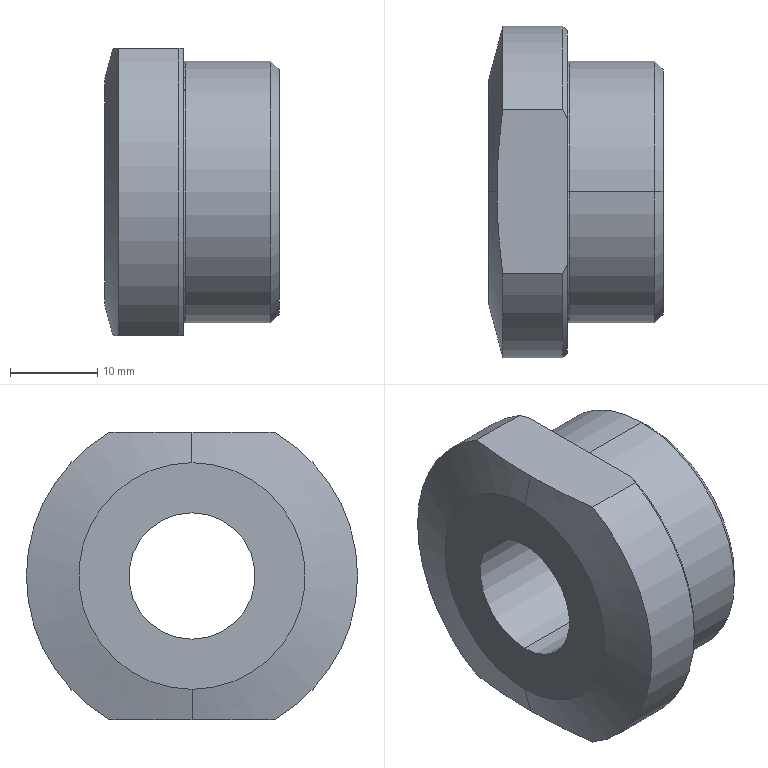Part | STEP file | Floating joint | 1 solid | 19 faces | box 20 x 38 x 33 mm | volume 13622 mm3 | cylinder 6 | cone 6 | plane 5 | torus 2 | commonest cylinder face diameters 14.5 x2 30 x2 38 x2
STEP:
#1=CARTESIAN_POINT('',(-9.,0.,7.25));
#2=VERTEX_POINT('',#1);
#3=CARTESIAN_POINT('',(-9.,0.,-7.25));
#4=VERTEX_POINT('',#3);
#5=CARTESIAN_POINT('',(-9.,0.,0.));
#6=DIRECTION('',(1.,0.,0.));
#7=DIRECTION('',(0.,0.,-1.));
#8=AXIS2_PLACEMENT_3D('',#5,#6,#7);
#9=CIRCLE('',#8,7.25);
#10=EDGE_CURVE('',#2,#4,#9,.T.);
#11=ORIENTED_EDGE('',*,*,#10,.F.);
#12=CARTESIAN_POINT('',(11.,0.,7.25));
#13=VERTEX_POINT('',#12);
#14=CARTESIAN_POINT('',(11.,0.,7.25));
#15=DIRECTION('',(1.,0.,0.));
#16=VECTOR('',#15,1000.);
#17=LINE('',#14,#16);
#18=EDGE_CURVE('',#2,#13,#17,.T.);
#19=ORIENTED_EDGE('',*,*,#18,.T.);
#20=CARTESIAN_POINT('',(11.,0.,-7.25));
#21=VERTEX_POINT('',#20);
#22=CARTESIAN_POINT('',(11.,0.,0.));
#23=DIRECTION('',(1.,0.,0.));
#24=DIRECTION('',(0.,0.,-1.));
#25=AXIS2_PLACEMENT_3D('',#22,#23,#24);
#26=CIRCLE('',#25,7.25);
#27=EDGE_CURVE('',#13,#21,#26,.T.);
#28=ORIENTED_EDGE('',*,*,#27,.T.);
#29=CARTESIAN_POINT('',(11.,0.,-7.25));
#30=DIRECTION('',(1.,0.,0.));
#31=VECTOR('',#30,1000.);
#32=LINE('',#29,#31);
#33=EDGE_CURVE('',#4,#21,#32,.T.);
#34=ORIENTED_EDGE('',*,*,#33,.F.);
#35=EDGE_LOOP('',(#11,#19,#28,#34));
#36=FACE_OUTER_BOUND('',#35,.T.);
#37=CARTESIAN_POINT('',(11.,0.,0.));
#38=DIRECTION('',(1.,0.,0.));
#39=DIRECTION('',(0.,0.,-1.));
#40=AXIS2_PLACEMENT_3D('',#37,#38,#39);
#41=CYLINDRICAL_SURFACE('',#40,7.25);
#42=ADVANCED_FACE('',(#36),#41,.F.);
#43=CARTESIAN_POINT('',(-9.,0.,0.));
#44=DIRECTION('',(1.,0.,0.));
#45=DIRECTION('',(0.,0.,-1.));
#46=AXIS2_PLACEMENT_3D('',#43,#44,#45);
#47=CIRCLE('',#46,7.25);
#48=EDGE_CURVE('',#4,#2,#47,.T.);
#49=ORIENTED_EDGE('',*,*,#48,.T.);
#50=ORIENTED_EDGE('',*,*,#10,.T.);
#51=EDGE_LOOP('',(#49,#50));
#52=FACE_BOUND('',#51,.T.);
#53=CARTESIAN_POINT('',(-9.,0.,-13.));
#54=VERTEX_POINT('',#53);
#55=CARTESIAN_POINT('',(-9.,0.,13.));
#56=VERTEX_POINT('',#55);
#57=CARTESIAN_POINT('',(-9.,0.,0.));
#58=DIRECTION('',(1.,0.,0.));
#59=DIRECTION('',(0.,0.,-1.));
#60=AXIS2_PLACEMENT_3D('',#57,#58,#59);
#61=CIRCLE('',#60,13.);
#62=EDGE_CURVE('',#54,#56,#61,.T.);
#63=ORIENTED_EDGE('',*,*,#62,.F.);
#64=CARTESIAN_POINT('',(-9.,0.,0.));
#65=DIRECTION('',(1.,0.,0.));
#66=DIRECTION('',(0.,0.,-1.));
#67=AXIS2_PLACEMENT_3D('',#64,#65,#66);
#68=CIRCLE('',#67,13.);
#69=EDGE_CURVE('',#56,#54,#68,.T.);
#70=ORIENTED_EDGE('',*,*,#69,.F.);
#71=EDGE_LOOP('',(#63,#70));
#72=FACE_OUTER_BOUND('',#71,.T.);
#73=CARTESIAN_POINT('',(-9.,0.,0.));
#74=DIRECTION('',(1.,0.,0.));
#75=DIRECTION('',(0.,0.,-1.));
#76=AXIS2_PLACEMENT_3D('',#73,#74,#75);
#77=PLANE('',#76);
#78=ADVANCED_FACE('',(#52,#72),#77,.F.);
#79=CARTESIAN_POINT('',(11.,0.,0.));
#80=DIRECTION('',(1.,0.,0.));
#81=DIRECTION('',(0.,0.,-1.));
#82=AXIS2_PLACEMENT_3D('',#79,#80,#81);
#83=CIRCLE('',#82,7.25);
#84=EDGE_CURVE('',#21,#13,#83,.T.);
#85=ORIENTED_EDGE('',*,*,#84,.F.);
#86=ORIENTED_EDGE('',*,*,#27,.F.);
#87=EDGE_LOOP('',(#85,#86));
#88=FACE_BOUND('',#87,.T.);
#89=CARTESIAN_POINT('',(11.,0.,-14.));
#90=VERTEX_POINT('',#89);
#91=CARTESIAN_POINT('',(11.,0.,14.));
#92=VERTEX_POINT('',#91);
#93=CARTESIAN_POINT('',(11.,0.,0.));
#94=DIRECTION('',(1.,0.,0.));
#95=DIRECTION('',(0.,0.,-1.));
#96=AXIS2_PLACEMENT_3D('',#93,#94,#95);
#97=CIRCLE('',#96,14.);
#98=EDGE_CURVE('',#90,#92,#97,.T.);
#99=ORIENTED_EDGE('',*,*,#98,.T.);
#100=CARTESIAN_POINT('',(11.,0.,0.));
#101=DIRECTION('',(1.,0.,0.));
#102=DIRECTION('',(0.,0.,-1.));
#103=AXIS2_PLACEMENT_3D('',#100,#101,#102);
#104=CIRCLE('',#103,14.);
#105=EDGE_CURVE('',#92,#90,#104,.T.);
#106=ORIENTED_EDGE('',*,*,#105,.T.);
#107=EDGE_LOOP('',(#99,#106));
#108=FACE_OUTER_BOUND('',#107,.T.);
#109=CARTESIAN_POINT('',(11.,14.,0.));
#110=DIRECTION('',(-1.,0.,0.));
#111=DIRECTION('',(0.,0.,1.));
#112=AXIS2_PLACEMENT_3D('',#109,#110,#111);
#113=PLANE('',#112);
#114=ADVANCED_FACE('',(#88,#108),#113,.F.);
#115=CARTESIAN_POINT('',(10.,0.,15.));
#116=VERTEX_POINT('',#115);
#117=CARTESIAN_POINT('',(10.,0.,-15.));
#118=VERTEX_POINT('',#117);
#119=CARTESIAN_POINT('',(10.,0.,0.));
#120=DIRECTION('',(1.,0.,0.));
#121=DIRECTION('',(0.,0.,-1.));
#122=AXIS2_PLACEMENT_3D('',#119,#120,#121);
#123=CIRCLE('',#122,15.);
#124=EDGE_CURVE('',#116,#118,#123,.T.);
#125=ORIENTED_EDGE('',*,*,#124,.T.);
#126=CARTESIAN_POINT('',(11.,0.,-14.));
#127=DIRECTION('',(-0.7071,0.,-0.7071));
#128=VECTOR('',#127,1000.);
#129=LINE('',#126,#128);
#130=EDGE_CURVE('',#90,#118,#129,.T.);
#131=ORIENTED_EDGE('',*,*,#130,.F.);
#132=ORIENTED_EDGE('',*,*,#105,.F.);
#133=CARTESIAN_POINT('',(11.,0.,14.));
#134=DIRECTION('',(-0.7071,0.,0.7071));
#135=VECTOR('',#134,1000.);
#136=LINE('',#133,#135);
#137=EDGE_CURVE('',#92,#116,#136,.T.);
#138=ORIENTED_EDGE('',*,*,#137,.T.);
#139=EDGE_LOOP('',(#125,#131,#132,#138));
#140=FACE_OUTER_BOUND('',#139,.T.);
#141=CARTESIAN_POINT('',(10.,0.,0.));
#142=DIRECTION('',(-1.,0.,0.));
#143=DIRECTION('',(0.,1.,0.));
#144=AXIS2_PLACEMENT_3D('',#141,#142,#143);
#145=CONICAL_SURFACE('',#144,15.,0.7854);
#146=ADVANCED_FACE('',(#140),#145,.T.);
#147=ORIENTED_EDGE('',*,*,#98,.F.);
#148=ORIENTED_EDGE('',*,*,#130,.T.);
#149=CARTESIAN_POINT('',(10.,0.,0.));
#150=DIRECTION('',(1.,0.,0.));
#151=DIRECTION('',(0.,0.,-1.));
#152=AXIS2_PLACEMENT_3D('',#149,#150,#151);
#153=CIRCLE('',#152,15.);
#154=EDGE_CURVE('',#118,#116,#153,.T.);
#155=ORIENTED_EDGE('',*,*,#154,.T.);
#156=ORIENTED_EDGE('',*,*,#137,.F.);
#157=EDGE_LOOP('',(#147,#148,#155,#156));
#158=FACE_OUTER_BOUND('',#157,.T.);
#159=CARTESIAN_POINT('',(10.,0.,0.));
#160=DIRECTION('',(-1.,0.,0.));
#161=DIRECTION('',(0.,-1.,0.));
#162=AXIS2_PLACEMENT_3D('',#159,#160,#161);
#163=CONICAL_SURFACE('',#162,15.,0.7854);
#164=ADVANCED_FACE('',(#158),#163,.T.);
#165=ORIENTED_EDGE('',*,*,#154,.F.);
#166=CARTESIAN_POINT('',(0.2,0.,-15.));
#167=VERTEX_POINT('',#166);
#168=CARTESIAN_POINT('',(10.,0.,-15.));
#169=DIRECTION('',(-1.,0.,0.));
#170=VECTOR('',#169,1000.);
#171=LINE('',#168,#170);
#172=EDGE_CURVE('',#118,#167,#171,.T.);
#173=ORIENTED_EDGE('',*,*,#172,.T.);
#174=CARTESIAN_POINT('',(0.2,0.,15.));
#175=VERTEX_POINT('',#174);
#176=CARTESIAN_POINT('',(0.2,0.,0.));
#177=DIRECTION('',(1.,0.,0.));
#178=DIRECTION('',(0.,0.,-1.));
#179=AXIS2_PLACEMENT_3D('',#176,#177,#178);
#180=CIRCLE('',#179,15.);
#181=EDGE_CURVE('',#167,#175,#180,.T.);
#182=ORIENTED_EDGE('',*,*,#181,.T.);
#183=CARTESIAN_POINT('',(10.,0.,15.));
#184=DIRECTION('',(-1.,0.,0.));
#185=VECTOR('',#184,1000.);
#186=LINE('',#183,#185);
#187=EDGE_CURVE('',#116,#175,#186,.T.);
#188=ORIENTED_EDGE('',*,*,#187,.F.);
#189=EDGE_LOOP('',(#165,#173,#182,#188));
#190=FACE_OUTER_BOUND('',#189,.T.);
#191=CARTESIAN_POINT('',(11.,0.,0.));
#192=DIRECTION('',(-1.,0.,0.));
#193=DIRECTION('',(0.,-1.,0.));
#194=AXIS2_PLACEMENT_3D('',#191,#192,#193);
#195=CYLINDRICAL_SURFACE('',#194,15.);
#196=ADVANCED_FACE('',(#190),#195,.T.);
#197=CARTESIAN_POINT('',(0.2,0.,0.));
#198=DIRECTION('',(1.,0.,0.));
#199=DIRECTION('',(0.,0.,-1.));
#200=AXIS2_PLACEMENT_3D('',#197,#198,#199);
#201=CIRCLE('',#200,15.);
#202=EDGE_CURVE('',#175,#167,#201,.T.);
#203=ORIENTED_EDGE('',*,*,#202,.T.);
#204=ORIENTED_EDGE('',*,*,#172,.F.);
#205=ORIENTED_EDGE('',*,*,#124,.F.);
#206=ORIENTED_EDGE('',*,*,#187,.T.);
#207=EDGE_LOOP('',(#203,#204,#205,#206));
#208=FACE_OUTER_BOUND('',#207,.T.);
#209=CARTESIAN_POINT('',(11.,0.,0.));
#210=DIRECTION('',(-1.,0.,0.));
#211=DIRECTION('',(0.,1.,0.));
#212=AXIS2_PLACEMENT_3D('',#209,#210,#211);
#213=CYLINDRICAL_SURFACE('',#212,15.);
#214=ADVANCED_FACE('',(#208),#213,.T.);
#215=ORIENTED_EDGE('',*,*,#202,.F.);
#216=CARTESIAN_POINT('',(0.,0.,15.2));
#217=VERTEX_POINT('',#216);
#218=CARTESIAN_POINT('',(0.2,0.,15.));
#219=CARTESIAN_POINT('',(0.1476,0.,15.));
#220=CARTESIAN_POINT('',(0.0956,0.,15.022));
#221=CARTESIAN_POINT('',(0.02155,0.,15.096));
#222=CARTESIAN_POINT('',(0.,0.,15.148));
#223=CARTESIAN_POINT('',(0.,0.,15.2));
#224=B_SPLINE_CURVE_WITH_KNOTS('',3,(#218,#219,#220,#221,#222,#223),.UNSPECIFIED.,.F.,.F.,(4,2,4),(0.,0.7854,1.571),.UNSPECIFIED.);
#225=EDGE_CURVE('',#175,#217,#224,.T.);
#226=ORIENTED_EDGE('',*,*,#225,.T.);
#227=CARTESIAN_POINT('',(0.,0.,-15.2));
#228=VERTEX_POINT('',#227);
#229=CARTESIAN_POINT('',(0.,0.,0.));
#230=DIRECTION('',(1.,0.,0.));
#231=DIRECTION('',(0.,0.,-1.));
#232=AXIS2_PLACEMENT_3D('',#229,#230,#231);
#233=CIRCLE('',#232,15.2);
#234=EDGE_CURVE('',#217,#228,#233,.T.);
#235=ORIENTED_EDGE('',*,*,#234,.T.);
#236=CARTESIAN_POINT('',(0.2,0.,-15.));
#237=CARTESIAN_POINT('',(0.1476,0.,-15.));
#238=CARTESIAN_POINT('',(0.0956,0.,-15.022));
#239=CARTESIAN_POINT('',(0.02155,0.,-15.096));
#240=CARTESIAN_POINT('',(0.,0.,-15.148));
#241=CARTESIAN_POINT('',(0.,0.,-15.2));
#242=B_SPLINE_CURVE_WITH_KNOTS('',3,(#236,#237,#238,#239,#240,#241),.UNSPECIFIED.,.F.,.F.,(4,2,4),(0.,0.7854,1.571),.UNSPECIFIED.);
#243=EDGE_CURVE('',#167,#228,#242,.T.);
#244=ORIENTED_EDGE('',*,*,#243,.F.);
#245=EDGE_LOOP('',(#215,#226,#235,#244));
#246=FACE_OUTER_BOUND('',#245,.T.);
#247=CARTESIAN_POINT('',(0.2,0.,0.));
#248=DIRECTION('',(1.,0.,0.));
#249=DIRECTION('',(0.,1.,0.));
#250=AXIS2_PLACEMENT_3D('',#247,#248,#249);
#251=TOROIDAL_SURFACE('',#250,15.2,0.2);
#252=ADVANCED_FACE('',(#246),#251,.F.);
#253=CARTESIAN_POINT('',(0.,0.,0.));
#254=DIRECTION('',(1.,0.,0.));
#255=DIRECTION('',(0.,0.,-1.));
#256=AXIS2_PLACEMENT_3D('',#253,#254,#255);
#257=CIRCLE('',#256,15.2);
#258=EDGE_CURVE('',#228,#217,#257,.T.);
#259=ORIENTED_EDGE('',*,*,#258,.T.);
#260=ORIENTED_EDGE('',*,*,#225,.F.);
#261=ORIENTED_EDGE('',*,*,#181,.F.);
#262=ORIENTED_EDGE('',*,*,#243,.T.);
#263=EDGE_LOOP('',(#259,#260,#261,#262));
#264=FACE_OUTER_BOUND('',#263,.T.);
#265=CARTESIAN_POINT('',(0.2,0.,0.));
#266=DIRECTION('',(1.,0.,0.));
#267=DIRECTION('',(0.,-1.,0.));
#268=AXIS2_PLACEMENT_3D('',#265,#266,#267);
#269=TOROIDAL_SURFACE('',#268,15.2,0.2);
#270=ADVANCED_FACE('',(#264),#269,.F.);
#271=ORIENTED_EDGE('',*,*,#258,.F.);
#272=ORIENTED_EDGE('',*,*,#234,.F.);
#273=EDGE_LOOP('',(#271,#272));
#274=FACE_BOUND('',#273,.T.);
#275=CARTESIAN_POINT('',(0.,-8.367,16.5));
#276=VERTEX_POINT('',#275);
#277=CARTESIAN_POINT('',(0.,8.367,16.5));
#278=VERTEX_POINT('',#277);
#279=CARTESIAN_POINT('',(0.,18.5,16.5));
#280=DIRECTION('',(0.,1.,0.));
#281=VECTOR('',#280,1000.);
#282=LINE('',#279,#281);
#283=EDGE_CURVE('',#276,#278,#282,.T.);
#284=ORIENTED_EDGE('',*,*,#283,.F.);
#285=CARTESIAN_POINT('',(0.,-8.367,-16.5));
#286=VERTEX_POINT('',#285);
#287=CARTESIAN_POINT('',(0.,0.,0.));
#288=DIRECTION('',(1.,0.,0.));
#289=DIRECTION('',(0.,0.,-1.));
#290=AXIS2_PLACEMENT_3D('',#287,#288,#289);
#291=CIRCLE('',#290,18.5);
#292=EDGE_CURVE('',#276,#286,#291,.T.);
#293=ORIENTED_EDGE('',*,*,#292,.T.);
#294=CARTESIAN_POINT('',(0.,8.367,-16.5));
#295=VERTEX_POINT('',#294);
#296=CARTESIAN_POINT('',(0.,18.5,-16.5));
#297=DIRECTION('',(0.,-1.,0.));
#298=VECTOR('',#297,1000.);
#299=LINE('',#296,#298);
#300=EDGE_CURVE('',#295,#286,#299,.T.);
#301=ORIENTED_EDGE('',*,*,#300,.F.);
#302=CARTESIAN_POINT('',(0.,0.,0.));
#303=DIRECTION('',(1.,0.,0.));
#304=DIRECTION('',(0.,0.,-1.));
#305=AXIS2_PLACEMENT_3D('',#302,#303,#304);
#306=CIRCLE('',#305,18.5);
#307=EDGE_CURVE('',#295,#278,#306,.T.);
#308=ORIENTED_EDGE('',*,*,#307,.T.);
#309=EDGE_LOOP('',(#284,#293,#301,#308));
#310=FACE_OUTER_BOUND('',#309,.T.);
#311=CARTESIAN_POINT('',(0.,18.5,0.));
#312=DIRECTION('',(-1.,0.,0.));
#313=DIRECTION('',(0.,0.,1.));
#314=AXIS2_PLACEMENT_3D('',#311,#312,#313);
#315=PLANE('',#314);
#316=ADVANCED_FACE('',(#274,#310),#315,.F.);
#317=CARTESIAN_POINT('',(-0.5,9.421,-16.5));
#318=VERTEX_POINT('',#317);
#319=CARTESIAN_POINT('',(-0.5,9.421,-16.5));
#320=CARTESIAN_POINT('',(-0.3272,9.072,-16.5));
#321=CARTESIAN_POINT('',(-0.1602,8.721,-16.5));
#322=CARTESIAN_POINT('',(0.,8.367,-16.5));
#323=B_SPLINE_CURVE_WITH_KNOTS('',3,(#319,#320,#321,#322),.UNSPECIFIED.,.F.,.F.,(4,4),(0.03698,0.03815),.UNSPECIFIED.);
#324=EDGE_CURVE('',#318,#295,#323,.T.);
#325=ORIENTED_EDGE('',*,*,#324,.F.);
#326=CARTESIAN_POINT('',(-0.5,9.421,16.5));
#327=VERTEX_POINT('',#326);
#328=CARTESIAN_POINT('',(-0.5,0.,0.));
#329=DIRECTION('',(1.,0.,0.));
#330=DIRECTION('',(0.,0.,-1.));
#331=AXIS2_PLACEMENT_3D('',#328,#329,#330);
#332=CIRCLE('',#331,19.);
#333=EDGE_CURVE('',#318,#327,#332,.T.);
#334=ORIENTED_EDGE('',*,*,#333,.T.);
#335=CARTESIAN_POINT('',(0.,8.367,16.5));
#336=CARTESIAN_POINT('',(-0.1605,8.722,16.5));
#337=CARTESIAN_POINT('',(-0.3275,9.073,16.5));
#338=CARTESIAN_POINT('',(-0.5,9.421,16.5));
#339=B_SPLINE_CURVE_WITH_KNOTS('',3,(#335,#336,#337,#338),.UNSPECIFIED.,.F.,.F.,(4,4),(0.05549,0.05666),.UNSPECIFIED.);
#340=EDGE_CURVE('',#278,#327,#339,.T.);
#341=ORIENTED_EDGE('',*,*,#340,.F.);
#342=ORIENTED_EDGE('',*,*,#307,.F.);
#343=EDGE_LOOP('',(#325,#334,#341,#342));
#344=FACE_OUTER_BOUND('',#343,.T.);
#345=CARTESIAN_POINT('',(-0.5,0.,0.));
#346=DIRECTION('',(-1.,0.,0.));
#347=DIRECTION('',(0.,-1.,0.));
#348=AXIS2_PLACEMENT_3D('',#345,#346,#347);
#349=CONICAL_SURFACE('',#348,19.,0.7854);
#350=ADVANCED_FACE('',(#344),#349,.T.);
#351=CARTESIAN_POINT('',(-0.5,-9.421,16.5));
#352=VERTEX_POINT('',#351);
#353=CARTESIAN_POINT('',(-0.5,-9.421,16.5));
#354=CARTESIAN_POINT('',(-0.3272,-9.072,16.5));
#355=CARTESIAN_POINT('',(-0.1602,-8.721,16.5));
#356=CARTESIAN_POINT('',(0.,-8.367,16.5));
#357=B_SPLINE_CURVE_WITH_KNOTS('',3,(#353,#354,#355,#356),.UNSPECIFIED.,.F.,.F.,(4,4),(0.03698,0.03815),.UNSPECIFIED.);
#358=EDGE_CURVE('',#352,#276,#357,.T.);
#359=ORIENTED_EDGE('',*,*,#358,.T.);
#360=ORIENTED_EDGE('',*,*,#283,.T.);
#361=ORIENTED_EDGE('',*,*,#340,.T.);
#362=CARTESIAN_POINT('',(-7.392,9.421,16.5));
#363=VERTEX_POINT('',#362);
#364=CARTESIAN_POINT('',(11.,9.421,16.5));
#365=DIRECTION('',(1.,0.,0.));
#366=VECTOR('',#365,1000.);
#367=LINE('',#364,#366);
#368=EDGE_CURVE('',#363,#327,#367,.T.);
#369=ORIENTED_EDGE('',*,*,#368,.F.);
#370=CARTESIAN_POINT('',(-8.062,0.,16.5));
#371=VERTEX_POINT('',#370);
#372=CARTESIAN_POINT('',(-8.062,0.,16.5));
#373=CARTESIAN_POINT('',(-8.062,1.573,16.5));
#374=CARTESIAN_POINT('',(-8.001,3.145,16.5));
#375=CARTESIAN_POINT('',(-7.77,6.285,16.5));
#376=CARTESIAN_POINT('',(-7.601,7.854,16.5));
#377=CARTESIAN_POINT('',(-7.392,9.421,16.5));
#378=B_SPLINE_CURVE_WITH_KNOTS('',3,(#372,#373,#374,#375,#376,#377),.UNSPECIFIED.,.F.,.F.,(4,2,4),(0.02541,0.03016,0.03491),.UNSPECIFIED.);
#379=EDGE_CURVE('',#371,#363,#378,.T.);
#380=ORIENTED_EDGE('',*,*,#379,.F.);
#381=CARTESIAN_POINT('',(-7.392,-9.421,16.5));
#382=VERTEX_POINT('',#381);
#383=CARTESIAN_POINT('',(-7.392,-9.421,16.5));
#384=CARTESIAN_POINT('',(-7.6,-7.856,16.5));
#385=CARTESIAN_POINT('',(-7.77,-6.28,16.5));
#386=CARTESIAN_POINT('',(-8.001,-3.138,16.5));
#387=CARTESIAN_POINT('',(-8.062,-1.568,16.5));
#388=CARTESIAN_POINT('',(-8.062,0.,16.5));
#389=B_SPLINE_CURVE_WITH_KNOTS('',3,(#383,#384,#385,#386,#387,#388),.UNSPECIFIED.,.F.,.F.,(4,2,4),(0.01595,0.02068,0.02541),.UNSPECIFIED.);
#390=EDGE_CURVE('',#382,#371,#389,.T.);
#391=ORIENTED_EDGE('',*,*,#390,.F.);
#392=CARTESIAN_POINT('',(11.,-9.421,16.5));
#393=DIRECTION('',(1.,0.,0.));
#394=VECTOR('',#393,1000.);
#395=LINE('',#392,#394);
#396=EDGE_CURVE('',#382,#352,#395,.T.);
#397=ORIENTED_EDGE('',*,*,#396,.T.);
#398=EDGE_LOOP('',(#359,#360,#361,#369,#380,#391,#397));
#399=FACE_OUTER_BOUND('',#398,.T.);
#400=CARTESIAN_POINT('',(0.,38.,16.5));
#401=DIRECTION('',(0.,0.,1.));
#402=DIRECTION('',(1.,0.,0.));
#403=AXIS2_PLACEMENT_3D('',#400,#401,#402);
#404=PLANE('',#403);
#405=ADVANCED_FACE('',(#399),#404,.T.);
#406=ORIENTED_EDGE('',*,*,#396,.F.);
#407=CARTESIAN_POINT('',(-7.392,-9.421,-16.5));
#408=VERTEX_POINT('',#407);
#409=CARTESIAN_POINT('',(-7.392,0.,0.));
#410=DIRECTION('',(1.,0.,0.));
#411=DIRECTION('',(0.,0.,-1.));
#412=AXIS2_PLACEMENT_3D('',#409,#410,#411);
#413=CIRCLE('',#412,19.);
#414=EDGE_CURVE('',#382,#408,#413,.T.);
#415=ORIENTED_EDGE('',*,*,#414,.T.);
#416=CARTESIAN_POINT('',(-0.5,-9.421,-16.5));
#417=VERTEX_POINT('',#416);
#418=CARTESIAN_POINT('',(11.,-9.421,-16.5));
#419=DIRECTION('',(1.,0.,0.));
#420=VECTOR('',#419,1000.);
#421=LINE('',#418,#420);
#422=EDGE_CURVE('',#408,#417,#421,.T.);
#423=ORIENTED_EDGE('',*,*,#422,.T.);
#424=CARTESIAN_POINT('',(-0.5,0.,0.));
#425=DIRECTION('',(1.,0.,0.));
#426=DIRECTION('',(0.,0.,-1.));
#427=AXIS2_PLACEMENT_3D('',#424,#425,#426);
#428=CIRCLE('',#427,19.);
#429=EDGE_CURVE('',#352,#417,#428,.T.);
#430=ORIENTED_EDGE('',*,*,#429,.F.);
#431=EDGE_LOOP('',(#406,#415,#423,#430));
#432=FACE_OUTER_BOUND('',#431,.T.);
#433=CARTESIAN_POINT('',(11.,0.,0.));
#434=DIRECTION('',(-1.,0.,0.));
#435=DIRECTION('',(0.,1.,0.));
#436=AXIS2_PLACEMENT_3D('',#433,#434,#435);
#437=CYLINDRICAL_SURFACE('',#436,19.);
#438=ADVANCED_FACE('',(#432),#437,.T.);
#439=ORIENTED_EDGE('',*,*,#358,.F.);
#440=ORIENTED_EDGE('',*,*,#429,.T.);
#441=CARTESIAN_POINT('',(0.,-8.367,-16.5));
#442=CARTESIAN_POINT('',(-0.1605,-8.722,-16.5));
#443=CARTESIAN_POINT('',(-0.3275,-9.073,-16.5));
#444=CARTESIAN_POINT('',(-0.5,-9.421,-16.5));
#445=B_SPLINE_CURVE_WITH_KNOTS('',3,(#441,#442,#443,#444),.UNSPECIFIED.,.F.,.F.,(4,4),(0.05549,0.05666),.UNSPECIFIED.);
#446=EDGE_CURVE('',#286,#417,#445,.T.);
#447=ORIENTED_EDGE('',*,*,#446,.F.);
#448=ORIENTED_EDGE('',*,*,#292,.F.);
#449=EDGE_LOOP('',(#439,#440,#447,#448));
#450=FACE_OUTER_BOUND('',#449,.T.);
#451=CARTESIAN_POINT('',(-0.5,0.,0.));
#452=DIRECTION('',(-1.,0.,0.));
#453=DIRECTION('',(0.,1.,0.));
#454=AXIS2_PLACEMENT_3D('',#451,#452,#453);
#455=CONICAL_SURFACE('',#454,19.,0.7854);
#456=ADVANCED_FACE('',(#450),#455,.T.);
#457=ORIENTED_EDGE('',*,*,#324,.T.);
#458=ORIENTED_EDGE('',*,*,#300,.T.);
#459=ORIENTED_EDGE('',*,*,#446,.T.);
#460=ORIENTED_EDGE('',*,*,#422,.F.);
#461=CARTESIAN_POINT('',(-8.062,0.,-16.5));
#462=VERTEX_POINT('',#461);
#463=CARTESIAN_POINT('',(-7.392,-9.421,-16.5));
#464=CARTESIAN_POINT('',(-7.6,-7.855,-16.5));
#465=CARTESIAN_POINT('',(-7.77,-6.28,-16.5));
#466=CARTESIAN_POINT('',(-8.001,-3.138,-16.5));
#467=CARTESIAN_POINT('',(-8.062,-1.568,-16.5));
#468=CARTESIAN_POINT('',(-8.062,0.,-16.5));
#469=B_SPLINE_CURVE_WITH_KNOTS('',3,(#463,#464,#465,#466,#467,#468),.UNSPECIFIED.,.F.,.F.,(4,2,4),(0.01595,0.02068,0.02541),.UNSPECIFIED.);
#470=EDGE_CURVE('',#408,#462,#469,.T.);
#471=ORIENTED_EDGE('',*,*,#470,.T.);
#472=CARTESIAN_POINT('',(-7.392,9.421,-16.5));
#473=VERTEX_POINT('',#472);
#474=CARTESIAN_POINT('',(-8.062,0.,-16.5));
#475=CARTESIAN_POINT('',(-8.062,1.573,-16.5));
#476=CARTESIAN_POINT('',(-8.001,3.145,-16.5));
#477=CARTESIAN_POINT('',(-7.77,6.285,-16.5));
#478=CARTESIAN_POINT('',(-7.601,7.854,-16.5));
#479=CARTESIAN_POINT('',(-7.392,9.421,-16.5));
#480=B_SPLINE_CURVE_WITH_KNOTS('',3,(#474,#475,#476,#477,#478,#479),.UNSPECIFIED.,.F.,.F.,(4,2,4),(0.02541,0.03016,0.03491),.UNSPECIFIED.);
#481=EDGE_CURVE('',#462,#473,#480,.T.);
#482=ORIENTED_EDGE('',*,*,#481,.T.);
#483=CARTESIAN_POINT('',(11.,9.421,-16.5));
#484=DIRECTION('',(1.,0.,0.));
#485=VECTOR('',#484,1000.);
#486=LINE('',#483,#485);
#487=EDGE_CURVE('',#473,#318,#486,.T.);
#488=ORIENTED_EDGE('',*,*,#487,.T.);
#489=EDGE_LOOP('',(#457,#458,#459,#460,#471,#482,#488));
#490=FACE_OUTER_BOUND('',#489,.T.);
#491=CARTESIAN_POINT('',(-10.8,38.,-16.5));
#492=DIRECTION('',(0.,0.,-1.));
#493=DIRECTION('',(-1.,0.,0.));
#494=AXIS2_PLACEMENT_3D('',#491,#492,#493);
#495=PLANE('',#494);
#496=ADVANCED_FACE('',(#490),#495,.T.);
#497=ORIENTED_EDGE('',*,*,#487,.F.);
#498=CARTESIAN_POINT('',(-7.392,0.,0.));
#499=DIRECTION('',(1.,0.,0.));
#500=DIRECTION('',(0.,0.,-1.));
#501=AXIS2_PLACEMENT_3D('',#498,#499,#500);
#502=CIRCLE('',#501,19.);
#503=EDGE_CURVE('',#473,#363,#502,.T.);
#504=ORIENTED_EDGE('',*,*,#503,.T.);
#505=ORIENTED_EDGE('',*,*,#368,.T.);
#506=ORIENTED_EDGE('',*,*,#333,.F.);
#507=EDGE_LOOP('',(#497,#504,#505,#506));
#508=FACE_OUTER_BOUND('',#507,.T.);
#509=CARTESIAN_POINT('',(11.,0.,0.));
#510=DIRECTION('',(-1.,0.,0.));
#511=DIRECTION('',(0.,-1.,0.));
#512=AXIS2_PLACEMENT_3D('',#509,#510,#511);
#513=CYLINDRICAL_SURFACE('',#512,19.);
#514=ADVANCED_FACE('',(#508),#513,.T.);
#515=ORIENTED_EDGE('',*,*,#379,.T.);
#516=ORIENTED_EDGE('',*,*,#503,.F.);
#517=ORIENTED_EDGE('',*,*,#481,.F.);
#518=CARTESIAN_POINT('',(-9.,0.,-13.));
#519=DIRECTION('',(0.2588,0.,-0.9659));
#520=VECTOR('',#519,1000.);
#521=LINE('',#518,#520);
#522=EDGE_CURVE('',#54,#462,#521,.T.);
#523=ORIENTED_EDGE('',*,*,#522,.F.);
#524=ORIENTED_EDGE('',*,*,#62,.T.);
#525=CARTESIAN_POINT('',(-9.,0.,13.));
#526=DIRECTION('',(0.2588,0.,0.9659));
#527=VECTOR('',#526,1000.);
#528=LINE('',#525,#527);
#529=EDGE_CURVE('',#56,#371,#528,.T.);
#530=ORIENTED_EDGE('',*,*,#529,.T.);
#531=EDGE_LOOP('',(#515,#516,#517,#523,#524,#530));
#532=FACE_OUTER_BOUND('',#531,.T.);
#533=CARTESIAN_POINT('',(-9.,0.,0.));
#534=DIRECTION('',(1.,0.,0.));
#535=DIRECTION('',(0.,-1.,0.));
#536=AXIS2_PLACEMENT_3D('',#533,#534,#535);
#537=CONICAL_SURFACE('',#536,13.,1.309);
#538=ADVANCED_FACE('',(#532),#537,.T.);
#539=ORIENTED_EDGE('',*,*,#69,.T.);
#540=ORIENTED_EDGE('',*,*,#522,.T.);
#541=ORIENTED_EDGE('',*,*,#470,.F.);
#542=ORIENTED_EDGE('',*,*,#414,.F.);
#543=ORIENTED_EDGE('',*,*,#390,.T.);
#544=ORIENTED_EDGE('',*,*,#529,.F.);
#545=EDGE_LOOP('',(#539,#540,#541,#542,#543,#544));
#546=FACE_OUTER_BOUND('',#545,.T.);
#547=CARTESIAN_POINT('',(-9.,0.,0.));
#548=DIRECTION('',(1.,0.,0.));
#549=DIRECTION('',(0.,1.,0.));
#550=AXIS2_PLACEMENT_3D('',#547,#548,#549);
#551=CONICAL_SURFACE('',#550,13.,1.309);
#552=ADVANCED_FACE('',(#546),#551,.T.);
#553=ORIENTED_EDGE('',*,*,#18,.F.);
#554=ORIENTED_EDGE('',*,*,#48,.F.);
#555=ORIENTED_EDGE('',*,*,#33,.T.);
#556=ORIENTED_EDGE('',*,*,#84,.T.);
#557=EDGE_LOOP('',(#553,#554,#555,#556));
#558=FACE_OUTER_BOUND('',#557,.T.);
#559=CARTESIAN_POINT('',(11.,0.,0.));
#560=DIRECTION('',(1.,0.,0.));
#561=DIRECTION('',(0.,0.,-1.));
#562=AXIS2_PLACEMENT_3D('',#559,#560,#561);
#563=CYLINDRICAL_SURFACE('',#562,7.25);
#564=ADVANCED_FACE('',(#558),#563,.F.);
#565=CLOSED_SHELL('',(#42,#78,#114,#146,#164,#196,#214,#252,#270,#316,#350,#405,#438,#456,#496,#514,#538,#552,#564));
#566=MANIFOLD_SOLID_BREP('',#565);
#567=CARTESIAN_POINT('',(0.,0.,0.));
#568=DIRECTION('',(0.,0.,1.));
#569=DIRECTION('',(1.,0.,0.));
#570=AXIS2_PLACEMENT_3D('',#567,#568,#569);
#571=(LENGTH_UNIT()NAMED_UNIT(*)SI_UNIT(.MILLI.,.METRE.));
#572=UNCERTAINTY_MEASURE_WITH_UNIT(LENGTH_MEASURE(0.00001),#571,'','');
#573=(NAMED_UNIT(*)PLANE_ANGLE_UNIT()SI_UNIT($,.RADIAN.));
#574=(NAMED_UNIT(*)SI_UNIT($,.STERADIAN.)SOLID_ANGLE_UNIT());
#575=(GEOMETRIC_REPRESENTATION_CONTEXT(3)GLOBAL_UNCERTAINTY_ASSIGNED_CONTEXT((#572))GLOBAL_UNIT_ASSIGNED_CONTEXT((#571,#573,#574))REPRESENTATION_CONTEXT('',''));
#576=ADVANCED_BREP_SHAPE_REPRESENTATION('',(#566,#570),#575);